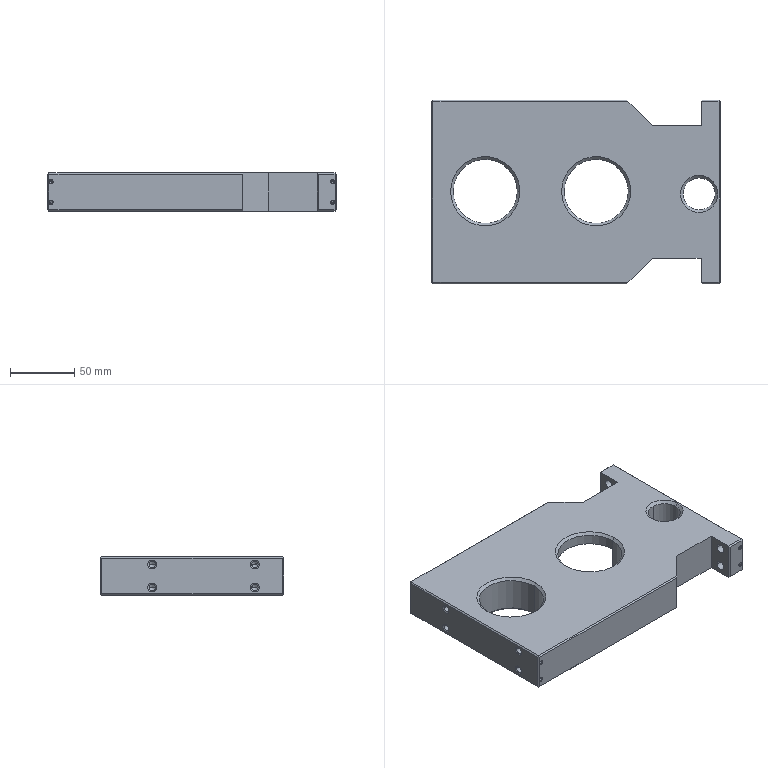Part | NX | 1 solid | 120 faces | box 225 x 143 x 30 mm | volume 671532 mm3 | cylinder 44 | cone 39 | plane 37 | commonest cylinder face diameters 5 x16 2.5 x12 7 x8 50 x4 10 x2 25 x2